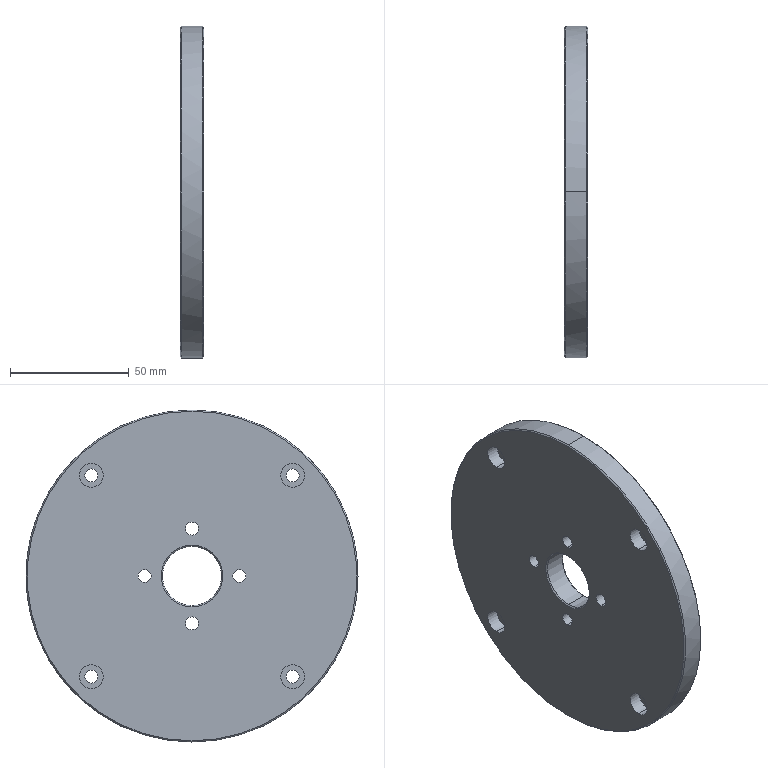Part | STEP file | 06-19 Stator fixing plate | 1 solid | 54 faces | box 10 x 140 x 140 mm | volume 144589 mm3 | cylinder 36 | plane 10 | cone 8 | commonest cylinder face diameters 5.5 x16 10 x16 25 x2 140 x2